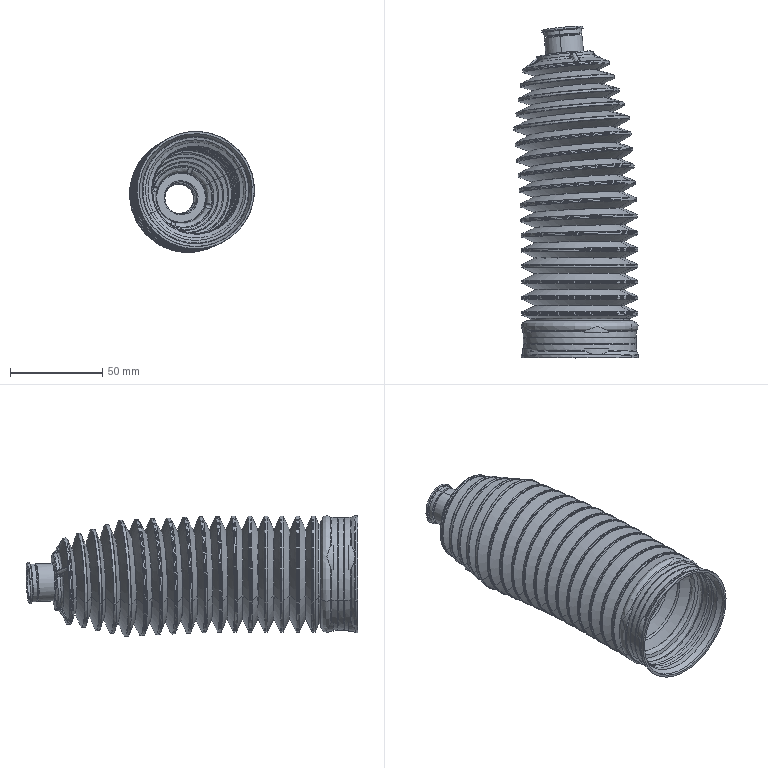Part | SolidWorks | features BaseBody 1 | 1 solid | 617 faces | box 67.591 x 179.747 x 65.54 mm | volume 46175 mm3 | spline 578 | plane 39